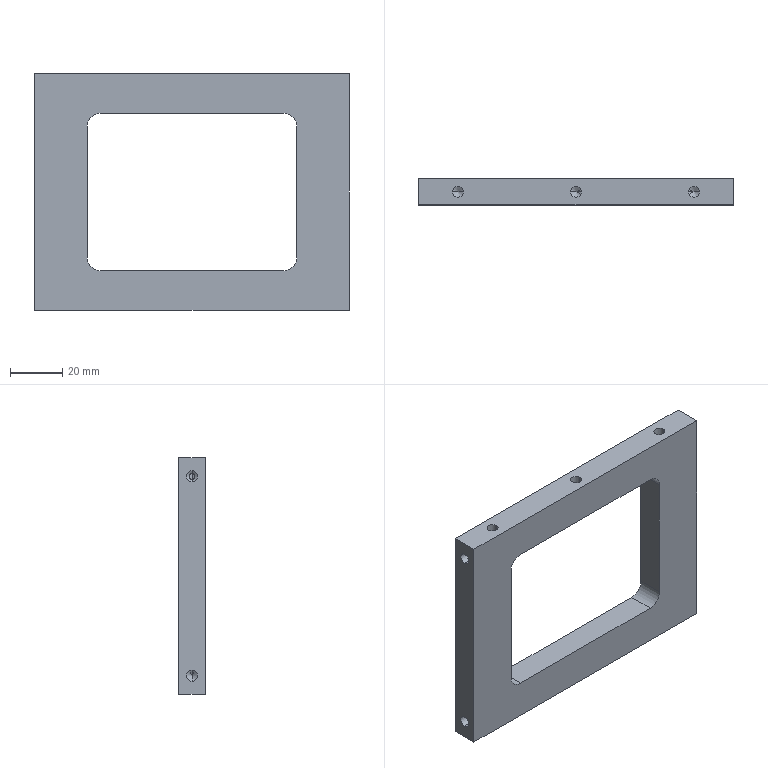Part | SolidWorks | features 3DProfileFeature 2, Cut 2, HoleWzd 2, Extrusion 1, ICE 1, MirrorPattern 1 | 1 solid | 42 faces | box 120 x 10 x 90 mm | volume 58973 mm3 | cylinder 18 | cone 14 | plane 10 | commonest cylinder face diameters 4.2 x14 10 x4
STEP:
#1=CARTESIAN_POINT('',(-45.,5.,31.338));
#2=VERTEX_POINT('',#1);
#3=CARTESIAN_POINT('',(-42.9,5.,32.6));
#4=VERTEX_POINT('',#3);
#5=CARTESIAN_POINT('',(-42.9,5.,32.6));
#6=DIRECTION('',(0.8572,0.,0.515));
#7=VECTOR('',#6,1000.);
#8=LINE('',#5,#7);
#9=EDGE_CURVE('',#2,#4,#8,.T.);
#10=ORIENTED_EDGE('',*,*,#9,.F.);
#11=CARTESIAN_POINT('',(-47.1,5.,32.6));
#12=VERTEX_POINT('',#11);
#13=CARTESIAN_POINT('',(-47.1,5.,32.6));
#14=DIRECTION('',(-0.8572,0.,0.515));
#15=VECTOR('',#14,1000.);
#16=LINE('',#13,#15);
#17=EDGE_CURVE('',#2,#12,#16,.T.);
#18=ORIENTED_EDGE('',*,*,#17,.T.);
#19=CARTESIAN_POINT('',(-45.,5.,32.6));
#20=DIRECTION('',(0.,0.,1.));
#21=DIRECTION('',(1.,0.,0.));
#22=AXIS2_PLACEMENT_3D('',#19,#20,#21);
#23=CIRCLE('',#22,2.1);
#24=EDGE_CURVE('',#12,#4,#23,.T.);
#25=ORIENTED_EDGE('',*,*,#24,.T.);
#26=EDGE_LOOP('',(#10,#18,#25));
#27=FACE_OUTER_BOUND('',#26,.T.);
#28=CARTESIAN_POINT('',(-45.,5.,32.6));
#29=DIRECTION('',(0.,0.,1.));
#30=DIRECTION('',(1.,0.,0.));
#31=AXIS2_PLACEMENT_3D('',#28,#29,#30);
#32=CONICAL_SURFACE('',#31,2.1,1.03);
#33=ADVANCED_FACE('',(#27),#32,.F.);
#34=ORIENTED_EDGE('',*,*,#24,.F.);
#35=CARTESIAN_POINT('',(-47.1,5.,36.732));
#36=VERTEX_POINT('',#35);
#37=CARTESIAN_POINT('',(-47.1,5.,45.));
#38=DIRECTION('',(0.,0.,1.));
#39=VECTOR('',#38,1000.);
#40=LINE('',#37,#39);
#41=EDGE_CURVE('',#12,#36,#40,.T.);
#42=ORIENTED_EDGE('',*,*,#41,.T.);
#43=CARTESIAN_POINT('',(-47.1,5.,39.268));
#44=VERTEX_POINT('',#43);
#45=CARTESIAN_POINT('',(-47.1,5.,39.268));
#46=CARTESIAN_POINT('',(-47.1,4.856,39.268));
#47=CARTESIAN_POINT('',(-47.084,4.712,39.214));
#48=CARTESIAN_POINT('',(-47.038,4.479,39.05));
#49=CARTESIAN_POINT('',(-47.009,4.383,38.94));
#50=CARTESIAN_POINT('',(-46.93,4.158,38.579));
#51=CARTESIAN_POINT('',(-46.889,4.083,38.287));
#52=CARTESIAN_POINT('',(-46.889,4.083,37.856));
#53=CARTESIAN_POINT('',(-46.899,4.102,37.71));
#54=CARTESIAN_POINT('',(-46.932,4.177,37.435));
#55=CARTESIAN_POINT('',(-46.956,4.233,37.301));
#56=CARTESIAN_POINT('',(-47.009,4.383,37.06));
#57=CARTESIAN_POINT('',(-47.038,4.478,36.95));
#58=CARTESIAN_POINT('',(-47.084,4.712,36.785));
#59=CARTESIAN_POINT('',(-47.1,4.856,36.732));
#60=CARTESIAN_POINT('',(-47.1,5.,36.732));
#61=B_SPLINE_CURVE_WITH_KNOTS('',3,(#45,#46,#47,#48,#49,#50,#51,#52,#53,#54,#55,#56,#57,#58,#59,#60),.UNSPECIFIED.,.F.,.F.,(4,2,2,2,2,2,2,4),(0.003814,0.004249,0.004683,0.005552,0.005986,0.00642,0.006854,0.007289),.UNSPECIFIED.);
#62=EDGE_CURVE('',#44,#36,#61,.T.);
#63=ORIENTED_EDGE('',*,*,#62,.F.);
#64=CARTESIAN_POINT('',(-47.1,5.,45.));
#65=VERTEX_POINT('',#64);
#66=CARTESIAN_POINT('',(-47.1,5.,45.));
#67=DIRECTION('',(0.,0.,1.));
#68=VECTOR('',#67,1000.);
#69=LINE('',#66,#68);
#70=EDGE_CURVE('',#44,#65,#69,.T.);
#71=ORIENTED_EDGE('',*,*,#70,.T.);
#72=CARTESIAN_POINT('',(-42.9,5.,45.));
#73=VERTEX_POINT('',#72);
#74=CARTESIAN_POINT('',(-45.,5.,45.));
#75=DIRECTION('',(0.,0.,1.));
#76=DIRECTION('',(1.,0.,0.));
#77=AXIS2_PLACEMENT_3D('',#74,#75,#76);
#78=CIRCLE('',#77,2.1);
#79=EDGE_CURVE('',#65,#73,#78,.T.);
#80=ORIENTED_EDGE('',*,*,#79,.T.);
#81=CARTESIAN_POINT('',(-42.9,5.,45.));
#82=DIRECTION('',(0.,0.,1.));
#83=VECTOR('',#82,1000.);
#84=LINE('',#81,#83);
#85=EDGE_CURVE('',#4,#73,#84,.T.);
#86=ORIENTED_EDGE('',*,*,#85,.F.);
#87=EDGE_LOOP('',(#34,#42,#63,#71,#80,#86));
#88=FACE_OUTER_BOUND('',#87,.T.);
#89=CARTESIAN_POINT('',(-45.,5.,45.));
#90=DIRECTION('',(0.,0.,1.));
#91=DIRECTION('',(1.,0.,0.));
#92=AXIS2_PLACEMENT_3D('',#89,#90,#91);
#93=CYLINDRICAL_SURFACE('',#92,2.1);
#94=ADVANCED_FACE('',(#88),#93,.F.);
#95=CARTESIAN_POINT('',(-2.1,5.,32.6));
#96=VERTEX_POINT('',#95);
#97=CARTESIAN_POINT('',(2.1,5.,32.6));
#98=VERTEX_POINT('',#97);
#99=CARTESIAN_POINT('',(0.,5.,32.6));
#100=DIRECTION('',(0.,0.,1.));
#101=DIRECTION('',(1.,0.,0.));
#102=AXIS2_PLACEMENT_3D('',#99,#100,#101);
#103=CIRCLE('',#102,2.1);
#104=EDGE_CURVE('',#96,#98,#103,.T.);
#105=ORIENTED_EDGE('',*,*,#104,.F.);
#106=CARTESIAN_POINT('',(-2.1,5.,45.));
#107=VERTEX_POINT('',#106);
#108=CARTESIAN_POINT('',(-2.1,5.,45.));
#109=DIRECTION('',(0.,0.,1.));
#110=VECTOR('',#109,1000.);
#111=LINE('',#108,#110);
#112=EDGE_CURVE('',#96,#107,#111,.T.);
#113=ORIENTED_EDGE('',*,*,#112,.T.);
#114=CARTESIAN_POINT('',(2.1,5.,45.));
#115=VERTEX_POINT('',#114);
#116=CARTESIAN_POINT('',(0.,5.,45.));
#117=DIRECTION('',(0.,0.,1.));
#118=DIRECTION('',(1.,0.,0.));
#119=AXIS2_PLACEMENT_3D('',#116,#117,#118);
#120=CIRCLE('',#119,2.1);
#121=EDGE_CURVE('',#107,#115,#120,.T.);
#122=ORIENTED_EDGE('',*,*,#121,.T.);
#123=CARTESIAN_POINT('',(2.1,5.,45.));
#124=DIRECTION('',(0.,0.,1.));
#125=VECTOR('',#124,1000.);
#126=LINE('',#123,#125);
#127=EDGE_CURVE('',#98,#115,#126,.T.);
#128=ORIENTED_EDGE('',*,*,#127,.F.);
#129=EDGE_LOOP('',(#105,#113,#122,#128));
#130=FACE_OUTER_BOUND('',#129,.T.);
#131=CARTESIAN_POINT('',(0.,5.,45.));
#132=DIRECTION('',(0.,0.,1.));
#133=DIRECTION('',(1.,0.,0.));
#134=AXIS2_PLACEMENT_3D('',#131,#132,#133);
#135=CYLINDRICAL_SURFACE('',#134,2.1);
#136=ADVANCED_FACE('',(#130),#135,.F.);
#137=CARTESIAN_POINT('',(0.,5.,31.338));
#138=VERTEX_POINT('',#137);
#139=CARTESIAN_POINT('',(2.1,5.,32.6));
#140=DIRECTION('',(0.8572,0.,0.515));
#141=VECTOR('',#140,1000.);
#142=LINE('',#139,#141);
#143=EDGE_CURVE('',#138,#98,#142,.T.);
#144=ORIENTED_EDGE('',*,*,#143,.F.);
#145=CARTESIAN_POINT('',(-2.1,5.,32.6));
#146=DIRECTION('',(-0.8572,0.,0.515));
#147=VECTOR('',#146,1000.);
#148=LINE('',#145,#147);
#149=EDGE_CURVE('',#138,#96,#148,.T.);
#150=ORIENTED_EDGE('',*,*,#149,.T.);
#151=ORIENTED_EDGE('',*,*,#104,.T.);
#152=EDGE_LOOP('',(#144,#150,#151));
#153=FACE_OUTER_BOUND('',#152,.T.);
#154=CARTESIAN_POINT('',(0.,5.,32.6));
#155=DIRECTION('',(0.,0.,1.));
#156=DIRECTION('',(1.,0.,0.));
#157=AXIS2_PLACEMENT_3D('',#154,#155,#156);
#158=CONICAL_SURFACE('',#157,2.1,1.03);
#159=ADVANCED_FACE('',(#153),#158,.F.);
#160=CARTESIAN_POINT('',(45.,5.,31.338));
#161=VERTEX_POINT('',#160);
#162=CARTESIAN_POINT('',(47.1,5.,32.6));
#163=VERTEX_POINT('',#162);
#164=CARTESIAN_POINT('',(47.1,5.,32.6));
#165=DIRECTION('',(0.8572,0.,0.515));
#166=VECTOR('',#165,1000.);
#167=LINE('',#164,#166);
#168=EDGE_CURVE('',#161,#163,#167,.T.);
#169=ORIENTED_EDGE('',*,*,#168,.F.);
#170=CARTESIAN_POINT('',(42.9,5.,32.6));
#171=VERTEX_POINT('',#170);
#172=CARTESIAN_POINT('',(42.9,5.,32.6));
#173=DIRECTION('',(-0.8572,0.,0.515));
#174=VECTOR('',#173,1000.);
#175=LINE('',#172,#174);
#176=EDGE_CURVE('',#161,#171,#175,.T.);
#177=ORIENTED_EDGE('',*,*,#176,.T.);
#178=CARTESIAN_POINT('',(45.,5.,32.6));
#179=DIRECTION('',(0.,0.,1.));
#180=DIRECTION('',(1.,0.,0.));
#181=AXIS2_PLACEMENT_3D('',#178,#179,#180);
#182=CIRCLE('',#181,2.1);
#183=EDGE_CURVE('',#171,#163,#182,.T.);
#184=ORIENTED_EDGE('',*,*,#183,.T.);
#185=EDGE_LOOP('',(#169,#177,#184));
#186=FACE_OUTER_BOUND('',#185,.T.);
#187=CARTESIAN_POINT('',(45.,5.,32.6));
#188=DIRECTION('',(0.,0.,1.));
#189=DIRECTION('',(1.,0.,0.));
#190=AXIS2_PLACEMENT_3D('',#187,#188,#189);
#191=CONICAL_SURFACE('',#190,2.1,1.03);
#192=ADVANCED_FACE('',(#186),#191,.F.);
#193=ORIENTED_EDGE('',*,*,#183,.F.);
#194=CARTESIAN_POINT('',(42.9,5.,45.));
#195=VERTEX_POINT('',#194);
#196=CARTESIAN_POINT('',(42.9,5.,45.));
#197=DIRECTION('',(0.,0.,1.));
#198=VECTOR('',#197,1000.);
#199=LINE('',#196,#198);
#200=EDGE_CURVE('',#171,#195,#199,.T.);
#201=ORIENTED_EDGE('',*,*,#200,.T.);
#202=CARTESIAN_POINT('',(47.1,5.,45.));
#203=VERTEX_POINT('',#202);
#204=CARTESIAN_POINT('',(45.,5.,45.));
#205=DIRECTION('',(0.,0.,1.));
#206=DIRECTION('',(1.,0.,0.));
#207=AXIS2_PLACEMENT_3D('',#204,#205,#206);
#208=CIRCLE('',#207,2.1);
#209=EDGE_CURVE('',#195,#203,#208,.T.);
#210=ORIENTED_EDGE('',*,*,#209,.T.);
#211=CARTESIAN_POINT('',(47.1,5.,39.268));
#212=VERTEX_POINT('',#211);
#213=CARTESIAN_POINT('',(47.1,5.,45.));
#214=DIRECTION('',(0.,0.,1.));
#215=VECTOR('',#214,1000.);
#216=LINE('',#213,#215);
#217=EDGE_CURVE('',#212,#203,#216,.T.);
#218=ORIENTED_EDGE('',*,*,#217,.F.);
#219=CARTESIAN_POINT('',(47.1,5.,36.732));
#220=VERTEX_POINT('',#219);
#221=CARTESIAN_POINT('',(47.1,5.,36.732));
#222=CARTESIAN_POINT('',(47.1,4.855,36.732));
#223=CARTESIAN_POINT('',(47.083,4.711,36.786));
#224=CARTESIAN_POINT('',(47.038,4.478,36.95));
#225=CARTESIAN_POINT('',(47.009,4.383,37.06));
#226=CARTESIAN_POINT('',(46.93,4.158,37.421));
#227=CARTESIAN_POINT('',(46.889,4.083,37.713));
#228=CARTESIAN_POINT('',(46.889,4.083,38.145));
#229=CARTESIAN_POINT('',(46.899,4.102,38.289));
#230=CARTESIAN_POINT('',(46.932,4.177,38.566));
#231=CARTESIAN_POINT('',(46.956,4.232,38.698));
#232=CARTESIAN_POINT('',(47.009,4.383,38.941));
#233=CARTESIAN_POINT('',(47.038,4.478,39.05));
#234=CARTESIAN_POINT('',(47.084,4.712,39.214));
#235=CARTESIAN_POINT('',(47.1,4.855,39.268));
#236=CARTESIAN_POINT('',(47.1,5.,39.268));
#237=B_SPLINE_CURVE_WITH_KNOTS('',3,(#221,#222,#223,#224,#225,#226,#227,#228,#229,#230,#231,#232,#233,#234,#235,#236),.UNSPECIFIED.,.F.,.F.,(4,2,2,2,2,2,2,4),(0.006577,0.007009,0.007441,0.008306,0.008738,0.00917,0.009602,0.01003),.UNSPECIFIED.);
#238=EDGE_CURVE('',#220,#212,#237,.T.);
#239=ORIENTED_EDGE('',*,*,#238,.F.);
#240=CARTESIAN_POINT('',(47.1,5.,45.));
#241=DIRECTION('',(0.,0.,1.));
#242=VECTOR('',#241,1000.);
#243=LINE('',#240,#242);
#244=EDGE_CURVE('',#163,#220,#243,.T.);
#245=ORIENTED_EDGE('',*,*,#244,.F.);
#246=EDGE_LOOP('',(#193,#201,#210,#218,#239,#245));
#247=FACE_OUTER_BOUND('',#246,.T.);
#248=CARTESIAN_POINT('',(45.,5.,45.));
#249=DIRECTION('',(0.,0.,1.));
#250=DIRECTION('',(1.,0.,0.));
#251=AXIS2_PLACEMENT_3D('',#248,#249,#250);
#252=CYLINDRICAL_SURFACE('',#251,2.1);
#253=ADVANCED_FACE('',(#247),#252,.F.);
#254=CARTESIAN_POINT('',(47.6,5.,40.1));
#255=VERTEX_POINT('',#254);
#256=CARTESIAN_POINT('',(47.6,5.,35.9));
#257=VERTEX_POINT('',#256);
#258=CARTESIAN_POINT('',(47.6,5.,38.));
#259=DIRECTION('',(1.,0.,0.));
#260=DIRECTION('',(0.,0.,-1.));
#261=AXIS2_PLACEMENT_3D('',#258,#259,#260);
#262=CIRCLE('',#261,2.1);
#263=EDGE_CURVE('',#255,#257,#262,.T.);
#264=ORIENTED_EDGE('',*,*,#263,.F.);
#265=CARTESIAN_POINT('',(60.,5.,40.1));
#266=VERTEX_POINT('',#265);
#267=CARTESIAN_POINT('',(60.,5.,40.1));
#268=DIRECTION('',(1.,0.,0.));
#269=VECTOR('',#268,1000.);
#270=LINE('',#267,#269);
#271=EDGE_CURVE('',#255,#266,#270,.T.);
#272=ORIENTED_EDGE('',*,*,#271,.T.);
#273=CARTESIAN_POINT('',(60.,5.,35.9));
#274=VERTEX_POINT('',#273);
#275=CARTESIAN_POINT('',(60.,5.,38.));
#276=DIRECTION('',(1.,0.,0.));
#277=DIRECTION('',(0.,0.,-1.));
#278=AXIS2_PLACEMENT_3D('',#275,#276,#277);
#279=CIRCLE('',#278,2.1);
#280=EDGE_CURVE('',#266,#274,#279,.T.);
#281=ORIENTED_EDGE('',*,*,#280,.T.);
#282=CARTESIAN_POINT('',(60.,5.,35.9));
#283=DIRECTION('',(1.,0.,0.));
#284=VECTOR('',#283,1000.);
#285=LINE('',#282,#284);
#286=EDGE_CURVE('',#257,#274,#285,.T.);
#287=ORIENTED_EDGE('',*,*,#286,.F.);
#288=EDGE_LOOP('',(#264,#272,#281,#287));
#289=FACE_OUTER_BOUND('',#288,.T.);
#290=CARTESIAN_POINT('',(60.,5.,38.));
#291=DIRECTION('',(1.,0.,0.));
#292=DIRECTION('',(0.,0.,-1.));
#293=AXIS2_PLACEMENT_3D('',#290,#291,#292);
#294=CYLINDRICAL_SURFACE('',#293,2.1);
#295=ADVANCED_FACE('',(#289),#294,.F.);
#296=ORIENTED_EDGE('',*,*,#238,.T.);
#297=CARTESIAN_POINT('',(47.6,5.,40.1));
#298=DIRECTION('',(0.515,0.,0.8572));
#299=VECTOR('',#298,1000.);
#300=LINE('',#297,#299);
#301=EDGE_CURVE('',#212,#255,#300,.T.);
#302=ORIENTED_EDGE('',*,*,#301,.T.);
#303=ORIENTED_EDGE('',*,*,#263,.T.);
#304=CARTESIAN_POINT('',(47.6,5.,35.9));
#305=DIRECTION('',(0.515,0.,-0.8572));
#306=VECTOR('',#305,1000.);
#307=LINE('',#304,#306);
#308=EDGE_CURVE('',#220,#257,#307,.T.);
#309=ORIENTED_EDGE('',*,*,#308,.F.);
#310=EDGE_LOOP('',(#296,#302,#303,#309));
#311=FACE_OUTER_BOUND('',#310,.T.);
#312=CARTESIAN_POINT('',(47.6,5.,38.));
#313=DIRECTION('',(1.,0.,0.));
#314=DIRECTION('',(0.,0.,-1.));
#315=AXIS2_PLACEMENT_3D('',#312,#313,#314);
#316=CONICAL_SURFACE('',#315,2.1,1.03);
#317=ADVANCED_FACE('',(#311),#316,.F.);
#318=CARTESIAN_POINT('',(47.6,5.,-35.9));
#319=VERTEX_POINT('',#318);
#320=CARTESIAN_POINT('',(47.6,5.,-40.1));
#321=VERTEX_POINT('',#320);
#322=CARTESIAN_POINT('',(47.6,5.,-38.));
#323=DIRECTION('',(1.,0.,0.));
#324=DIRECTION('',(0.,0.,-1.));
#325=AXIS2_PLACEMENT_3D('',#322,#323,#324);
#326=CIRCLE('',#325,2.1);
#327=EDGE_CURVE('',#319,#321,#326,.T.);
#328=ORIENTED_EDGE('',*,*,#327,.F.);
#329=CARTESIAN_POINT('',(60.,5.,-35.9));
#330=VERTEX_POINT('',#329);
#331=CARTESIAN_POINT('',(60.,5.,-35.9));
#332=DIRECTION('',(1.,0.,0.));
#333=VECTOR('',#332,1000.);
#334=LINE('',#331,#333);
#335=EDGE_CURVE('',#319,#330,#334,.T.);
#336=ORIENTED_EDGE('',*,*,#335,.T.);
#337=CARTESIAN_POINT('',(60.,5.,-40.1));
#338=VERTEX_POINT('',#337);
#339=CARTESIAN_POINT('',(60.,5.,-38.));
#340=DIRECTION('',(1.,0.,0.));
#341=DIRECTION('',(0.,0.,-1.));
#342=AXIS2_PLACEMENT_3D('',#339,#340,#341);
#343=CIRCLE('',#342,2.1);
#344=EDGE_CURVE('',#330,#338,#343,.T.);
#345=ORIENTED_EDGE('',*,*,#344,.T.);
#346=CARTESIAN_POINT('',(60.,5.,-40.1));
#347=DIRECTION('',(1.,0.,0.));
#348=VECTOR('',#347,1000.);
#349=LINE('',#346,#348);
#350=EDGE_CURVE('',#321,#338,#349,.T.);
#351=ORIENTED_EDGE('',*,*,#350,.F.);
#352=EDGE_LOOP('',(#328,#336,#345,#351));
#353=FACE_OUTER_BOUND('',#352,.T.);
#354=CARTESIAN_POINT('',(60.,5.,-38.));
#355=DIRECTION('',(1.,0.,0.));
#356=DIRECTION('',(0.,0.,-1.));
#357=AXIS2_PLACEMENT_3D('',#354,#355,#356);
#358=CYLINDRICAL_SURFACE('',#357,2.1);
#359=ADVANCED_FACE('',(#353),#358,.F.);
#360=CARTESIAN_POINT('',(46.338,5.,-38.));
#361=VERTEX_POINT('',#360);
#362=CARTESIAN_POINT('',(47.6,5.,-40.1));
#363=DIRECTION('',(0.515,0.,-0.8572));
#364=VECTOR('',#363,1000.);
#365=LINE('',#362,#364);
#366=EDGE_CURVE('',#361,#321,#365,.T.);
#367=ORIENTED_EDGE('',*,*,#366,.F.);
#368=CARTESIAN_POINT('',(47.6,5.,-35.9));
#369=DIRECTION('',(0.515,0.,0.8572));
#370=VECTOR('',#369,1000.);
#371=LINE('',#368,#370);
#372=EDGE_CURVE('',#361,#319,#371,.T.);
#373=ORIENTED_EDGE('',*,*,#372,.T.);
#374=ORIENTED_EDGE('',*,*,#327,.T.);
#375=EDGE_LOOP('',(#367,#373,#374));
#376=FACE_OUTER_BOUND('',#375,.T.);
#377=CARTESIAN_POINT('',(47.6,5.,-38.));
#378=DIRECTION('',(1.,0.,0.));
#379=DIRECTION('',(0.,0.,-1.));
#380=AXIS2_PLACEMENT_3D('',#377,#378,#379);
#381=CONICAL_SURFACE('',#380,2.1,1.03);
#382=ADVANCED_FACE('',(#376),#381,.F.);
#383=CARTESIAN_POINT('',(-47.6,5.,35.9));
#384=VERTEX_POINT('',#383);
#385=CARTESIAN_POINT('',(-47.6,5.,40.1));
#386=VERTEX_POINT('',#385);
#387=CARTESIAN_POINT('',(-47.6,5.,38.));
#388=DIRECTION('',(-1.,0.,0.));
#389=DIRECTION('',(0.,0.,1.));
#390=AXIS2_PLACEMENT_3D('',#387,#388,#389);
#391=CIRCLE('',#390,2.1);
#392=EDGE_CURVE('',#384,#386,#391,.T.);
#393=ORIENTED_EDGE('',*,*,#392,.F.);
#394=CARTESIAN_POINT('',(-60.,5.,35.9));
#395=VERTEX_POINT('',#394);
#396=CARTESIAN_POINT('',(-60.,5.,35.9));
#397=DIRECTION('',(-1.,0.,0.));
#398=VECTOR('',#397,1000.);
#399=LINE('',#396,#398);
#400=EDGE_CURVE('',#384,#395,#399,.T.);
#401=ORIENTED_EDGE('',*,*,#400,.T.);
#402=CARTESIAN_POINT('',(-60.,5.,40.1));
#403=VERTEX_POINT('',#402);
#404=CARTESIAN_POINT('',(-60.,5.,38.));
#405=DIRECTION('',(-1.,0.,0.));
#406=DIRECTION('',(0.,0.,1.));
#407=AXIS2_PLACEMENT_3D('',#404,#405,#406);
#408=CIRCLE('',#407,2.1);
#409=EDGE_CURVE('',#395,#403,#408,.T.);
#410=ORIENTED_EDGE('',*,*,#409,.T.);
#411=CARTESIAN_POINT('',(-60.,5.,40.1));
#412=DIRECTION('',(-1.,0.,0.));
#413=VECTOR('',#412,1000.);
#414=LINE('',#411,#413);
#415=EDGE_CURVE('',#386,#403,#414,.T.);
#416=ORIENTED_EDGE('',*,*,#415,.F.);
#417=EDGE_LOOP('',(#393,#401,#410,#416));
#418=FACE_OUTER_BOUND('',#417,.T.);
#419=CARTESIAN_POINT('',(-60.,5.,38.));
#420=DIRECTION('',(-1.,0.,0.));
#421=DIRECTION('',(0.,0.,1.));
#422=AXIS2_PLACEMENT_3D('',#419,#420,#421);
#423=CYLINDRICAL_SURFACE('',#422,2.1);
#424=ADVANCED_FACE('',(#418),#423,.F.);
#425=ORIENTED_EDGE('',*,*,#62,.T.);
#426=CARTESIAN_POINT('',(-47.6,5.,35.9));
#427=DIRECTION('',(-0.515,0.,-0.8572));
#428=VECTOR('',#427,1000.);
#429=LINE('',#426,#428);
#430=EDGE_CURVE('',#36,#384,#429,.T.);
#431=ORIENTED_EDGE('',*,*,#430,.T.);
#432=ORIENTED_EDGE('',*,*,#392,.T.);
#433=CARTESIAN_POINT('',(-47.6,5.,40.1));
#434=DIRECTION('',(-0.515,0.,0.8572));
#435=VECTOR('',#434,1000.);
#436=LINE('',#433,#435);
#437=EDGE_CURVE('',#44,#386,#436,.T.);
#438=ORIENTED_EDGE('',*,*,#437,.F.);
#439=EDGE_LOOP('',(#425,#431,#432,#438));
#440=FACE_OUTER_BOUND('',#439,.T.);
#441=CARTESIAN_POINT('',(-47.6,5.,38.));
#442=DIRECTION('',(-1.,0.,0.));
#443=DIRECTION('',(0.,0.,1.));
#444=AXIS2_PLACEMENT_3D('',#441,#442,#443);
#445=CONICAL_SURFACE('',#444,2.1,1.03);
#446=ADVANCED_FACE('',(#440),#445,.F.);
#447=CARTESIAN_POINT('',(-47.6,5.,-40.1));
#448=VERTEX_POINT('',#447);
#449=CARTESIAN_POINT('',(-47.6,5.,-35.9));
#450=VERTEX_POINT('',#449);
#451=CARTESIAN_POINT('',(-47.6,5.,-38.));
#452=DIRECTION('',(-1.,0.,0.));
#453=DIRECTION('',(0.,0.,1.));
#454=AXIS2_PLACEMENT_3D('',#451,#452,#453);
#455=CIRCLE('',#454,2.1);
#456=EDGE_CURVE('',#448,#450,#455,.T.);
#457=ORIENTED_EDGE('',*,*,#456,.F.);
#458=CARTESIAN_POINT('',(-60.,5.,-40.1));
#459=VERTEX_POINT('',#458);
#460=CARTESIAN_POINT('',(-60.,5.,-40.1));
#461=DIRECTION('',(-1.,0.,0.));
#462=VECTOR('',#461,1000.);
#463=LINE('',#460,#462);
#464=EDGE_CURVE('',#448,#459,#463,.T.);
#465=ORIENTED_EDGE('',*,*,#464,.T.);
#466=CARTESIAN_POINT('',(-60.,5.,-35.9));
#467=VERTEX_POINT('',#466);
#468=CARTESIAN_POINT('',(-60.,5.,-38.));
#469=DIRECTION('',(-1.,0.,0.));
#470=DIRECTION('',(0.,0.,1.));
#471=AXIS2_PLACEMENT_3D('',#468,#469,#470);
#472=CIRCLE('',#471,2.1);
#473=EDGE_CURVE('',#459,#467,#472,.T.);
#474=ORIENTED_EDGE('',*,*,#473,.T.);
#475=CARTESIAN_POINT('',(-60.,5.,-35.9));
#476=DIRECTION('',(-1.,0.,0.));
#477=VECTOR('',#476,1000.);
#478=LINE('',#475,#477);
#479=EDGE_CURVE('',#450,#467,#478,.T.);
#480=ORIENTED_EDGE('',*,*,#479,.F.);
#481=EDGE_LOOP('',(#457,#465,#474,#480));
#482=FACE_OUTER_BOUND('',#481,.T.);
#483=CARTESIAN_POINT('',(-60.,5.,-38.));
#484=DIRECTION('',(-1.,0.,0.));
#485=DIRECTION('',(0.,0.,1.));
#486=AXIS2_PLACEMENT_3D('',#483,#484,#485);
#487=CYLINDRICAL_SURFACE('',#486,2.1);
#488=ADVANCED_FACE('',(#482),#487,.F.);
#489=CARTESIAN_POINT('',(-46.338,5.,-38.));
#490=VERTEX_POINT('',#489);
#491=CARTESIAN_POINT('',(-47.6,5.,-35.9));
#492=DIRECTION('',(-0.515,0.,0.8572));
#493=VECTOR('',#492,1000.);
#494=LINE('',#491,#493);
#495=EDGE_CURVE('',#490,#450,#494,.T.);
#496=ORIENTED_EDGE('',*,*,#495,.F.);
#497=CARTESIAN_POINT('',(-47.6,5.,-40.1));
#498=DIRECTION('',(-0.515,0.,-0.8572));
#499=VECTOR('',#498,1000.);
#500=LINE('',#497,#499);
#501=EDGE_CURVE('',#490,#448,#500,.T.);
#502=ORIENTED_EDGE('',*,*,#501,.T.);
#503=ORIENTED_EDGE('',*,*,#456,.T.);
#504=EDGE_LOOP('',(#496,#502,#503));
#505=FACE_OUTER_BOUND('',#504,.T.);
#506=CARTESIAN_POINT('',(-47.6,5.,-38.));
#507=DIRECTION('',(-1.,0.,0.));
#508=DIRECTION('',(0.,0.,1.));
#509=AXIS2_PLACEMENT_3D('',#506,#507,#508);
#510=CONICAL_SURFACE('',#509,2.1,1.03);
#511=ADVANCED_FACE('',(#505),#510,.F.);
#512=CARTESIAN_POINT('',(60.,5.,38.));
#513=DIRECTION('',(1.,0.,0.));
#514=DIRECTION('',(0.,0.,-1.));
#515=AXIS2_PLACEMENT_3D('',#512,#513,#514);
#516=CIRCLE('',#515,2.1);
#517=EDGE_CURVE('',#274,#266,#516,.T.);
#518=ORIENTED_EDGE('',*,*,#517,.F.);
#519=ORIENTED_EDGE('',*,*,#280,.F.);
#520=EDGE_LOOP('',(#518,#519));
#521=FACE_BOUND('',#520,.T.);
#522=CARTESIAN_POINT('',(60.,5.,-38.));
#523=DIRECTION('',(1.,0.,0.));
#524=DIRECTION('',(0.,0.,-1.));
#525=AXIS2_PLACEMENT_3D('',#522,#523,#524);
#526=CIRCLE('',#525,2.1);
#527=EDGE_CURVE('',#338,#330,#526,.T.);
#528=ORIENTED_EDGE('',*,*,#527,.F.);
#529=ORIENTED_EDGE('',*,*,#344,.F.);
#530=EDGE_LOOP('',(#528,#529));
#531=FACE_BOUND('',#530,.T.);
#532=CARTESIAN_POINT('',(60.,0.,45.));
#533=VERTEX_POINT('',#532);
#534=CARTESIAN_POINT('',(60.,0.,-45.));
#535=VERTEX_POINT('',#534);
#536=CARTESIAN_POINT('',(60.,0.,-45.));
#537=DIRECTION('',(0.,0.,-1.));
#538=VECTOR('',#537,1000.);
#539=LINE('',#536,#538);
#540=EDGE_CURVE('',#533,#535,#539,.T.);
#541=ORIENTED_EDGE('',*,*,#540,.T.);
#542=CARTESIAN_POINT('',(60.,10.,-45.));
#543=VERTEX_POINT('',#542);
#544=CARTESIAN_POINT('',(60.,10.,-45.));
#545=DIRECTION('',(0.,-1.,0.));
#546=VECTOR('',#545,1000.);
#547=LINE('',#544,#546);
#548=EDGE_CURVE('',#543,#535,#547,.T.);
#549=ORIENTED_EDGE('',*,*,#548,.F.);
#550=CARTESIAN_POINT('',(60.,10.,45.));
#551=VERTEX_POINT('',#550);
#552=CARTESIAN_POINT('',(60.,10.,-45.));
#553=DIRECTION('',(0.,0.,-1.));
#554=VECTOR('',#553,1000.);
#555=LINE('',#552,#554);
#556=EDGE_CURVE('',#551,#543,#555,.T.);
#557=ORIENTED_EDGE('',*,*,#556,.F.);
#558=CARTESIAN_POINT('',(60.,10.,45.));
#559=DIRECTION('',(0.,-1.,0.));
#560=VECTOR('',#559,1000.);
#561=LINE('',#558,#560);
#562=EDGE_CURVE('',#551,#533,#561,.T.);
#563=ORIENTED_EDGE('',*,*,#562,.T.);
#564=EDGE_LOOP('',(#541,#549,#557,#563));
#565=FACE_OUTER_BOUND('',#564,.T.);
#566=CARTESIAN_POINT('',(60.,10.,-45.));
#567=DIRECTION('',(-1.,0.,0.));
#568=DIRECTION('',(0.,0.,1.));
#569=AXIS2_PLACEMENT_3D('',#566,#567,#568);
#570=PLANE('',#569);
#571=ADVANCED_FACE('',(#521,#531,#565),#570,.F.);
#572=CARTESIAN_POINT('',(-60.,0.,-45.));
#573=VERTEX_POINT('',#572);
#574=CARTESIAN_POINT('',(-60.,0.,-45.));
#575=DIRECTION('',(-1.,0.,0.));
#576=VECTOR('',#575,1000.);
#577=LINE('',#574,#576);
#578=EDGE_CURVE('',#535,#573,#577,.T.);
#579=ORIENTED_EDGE('',*,*,#578,.T.);
#580=CARTESIAN_POINT('',(-60.,10.,-45.));
#581=VERTEX_POINT('',#580);
#582=CARTESIAN_POINT('',(-60.,10.,-45.));
#583=DIRECTION('',(0.,-1.,0.));
#584=VECTOR('',#583,1000.);
#585=LINE('',#582,#584);
#586=EDGE_CURVE('',#581,#573,#585,.T.);
#587=ORIENTED_EDGE('',*,*,#586,.F.);
#588=CARTESIAN_POINT('',(-60.,10.,-45.));
#589=DIRECTION('',(-1.,0.,0.));
#590=VECTOR('',#589,1000.);
#591=LINE('',#588,#590);
#592=EDGE_CURVE('',#543,#581,#591,.T.);
#593=ORIENTED_EDGE('',*,*,#592,.F.);
#594=ORIENTED_EDGE('',*,*,#548,.T.);
#595=EDGE_LOOP('',(#579,#587,#593,#594));
#596=FACE_OUTER_BOUND('',#595,.T.);
#597=CARTESIAN_POINT('',(-60.,10.,-45.));
#598=DIRECTION('',(0.,0.,1.));
#599=DIRECTION('',(1.,0.,0.));
#600=AXIS2_PLACEMENT_3D('',#597,#598,#599);
#601=PLANE('',#600);
#602=ADVANCED_FACE('',(#596),#601,.F.);
#603=CARTESIAN_POINT('',(-60.,5.,38.));
#604=DIRECTION('',(-1.,0.,0.));
#605=DIRECTION('',(0.,0.,1.));
#606=AXIS2_PLACEMENT_3D('',#603,#604,#605);
#607=CIRCLE('',#606,2.1);
#608=EDGE_CURVE('',#403,#395,#607,.T.);
#609=ORIENTED_EDGE('',*,*,#608,.F.);
#610=ORIENTED_EDGE('',*,*,#409,.F.);
#611=EDGE_LOOP('',(#609,#610));
#612=FACE_BOUND('',#611,.T.);
#613=CARTESIAN_POINT('',(-60.,5.,-38.));
#614=DIRECTION('',(-1.,0.,0.));
#615=DIRECTION('',(0.,0.,1.));
#616=AXIS2_PLACEMENT_3D('',#613,#614,#615);
#617=CIRCLE('',#616,2.1);
#618=EDGE_CURVE('',#467,#459,#617,.T.);
#619=ORIENTED_EDGE('',*,*,#618,.F.);
#620=ORIENTED_EDGE('',*,*,#473,.F.);
#621=EDGE_LOOP('',(#619,#620));
#622=FACE_BOUND('',#621,.T.);
#623=CARTESIAN_POINT('',(-60.,0.,45.));
#624=VERTEX_POINT('',#623);
#625=CARTESIAN_POINT('',(-60.,0.,-45.));
#626=DIRECTION('',(0.,0.,1.));
#627=VECTOR('',#626,1000.);
#628=LINE('',#625,#627);
#629=EDGE_CURVE('',#573,#624,#628,.T.);
#630=ORIENTED_EDGE('',*,*,#629,.T.);
#631=CARTESIAN_POINT('',(-60.,10.,45.));
#632=VERTEX_POINT('',#631);
#633=CARTESIAN_POINT('',(-60.,10.,45.));
#634=DIRECTION('',(0.,-1.,0.));
#635=VECTOR('',#634,1000.);
#636=LINE('',#633,#635);
#637=EDGE_CURVE('',#632,#624,#636,.T.);
#638=ORIENTED_EDGE('',*,*,#637,.F.);
#639=CARTESIAN_POINT('',(-60.,10.,-45.));
#640=DIRECTION('',(0.,0.,1.));
#641=VECTOR('',#640,1000.);
#642=LINE('',#639,#641);
#643=EDGE_CURVE('',#581,#632,#642,.T.);
#644=ORIENTED_EDGE('',*,*,#643,.F.);
#645=ORIENTED_EDGE('',*,*,#586,.T.);
#646=EDGE_LOOP('',(#630,#638,#644,#645));
#647=FACE_OUTER_BOUND('',#646,.T.);
#648=CARTESIAN_POINT('',(-60.,10.,-45.));
#649=DIRECTION('',(1.,0.,0.));
#650=DIRECTION('',(0.,0.,-1.));
#651=AXIS2_PLACEMENT_3D('',#648,#649,#650);
#652=PLANE('',#651);
#653=ADVANCED_FACE('',(#612,#622,#647),#652,.F.);
#654=CARTESIAN_POINT('',(-45.,5.,45.));
#655=DIRECTION('',(0.,0.,1.));
#656=DIRECTION('',(1.,0.,0.));
#657=AXIS2_PLACEMENT_3D('',#654,#655,#656);
#658=CIRCLE('',#657,2.1);
#659=EDGE_CURVE('',#73,#65,#658,.T.);
#660=ORIENTED_EDGE('',*,*,#659,.F.);
#661=ORIENTED_EDGE('',*,*,#79,.F.);
#662=EDGE_LOOP('',(#660,#661));
#663=FACE_BOUND('',#662,.T.);
#664=CARTESIAN_POINT('',(0.,5.,45.));
#665=DIRECTION('',(0.,0.,1.));
#666=DIRECTION('',(1.,0.,0.));
#667=AXIS2_PLACEMENT_3D('',#664,#665,#666);
#668=CIRCLE('',#667,2.1);
#669=EDGE_CURVE('',#115,#107,#668,.T.);
#670=ORIENTED_EDGE('',*,*,#669,.F.);
#671=ORIENTED_EDGE('',*,*,#121,.F.);
#672=EDGE_LOOP('',(#670,#671));
#673=FACE_BOUND('',#672,.T.);
#674=CARTESIAN_POINT('',(45.,5.,45.));
#675=DIRECTION('',(0.,0.,1.));
#676=DIRECTION('',(1.,0.,0.));
#677=AXIS2_PLACEMENT_3D('',#674,#675,#676);
#678=CIRCLE('',#677,2.1);
#679=EDGE_CURVE('',#203,#195,#678,.T.);
#680=ORIENTED_EDGE('',*,*,#679,.F.);
#681=ORIENTED_EDGE('',*,*,#209,.F.);
#682=EDGE_LOOP('',(#680,#681));
#683=FACE_BOUND('',#682,.T.);
#684=CARTESIAN_POINT('',(-60.,0.,45.));
#685=DIRECTION('',(1.,0.,0.));
#686=VECTOR('',#685,1000.);
#687=LINE('',#684,#686);
#688=EDGE_CURVE('',#624,#533,#687,.T.);
#689=ORIENTED_EDGE('',*,*,#688,.T.);
#690=ORIENTED_EDGE('',*,*,#562,.F.);
#691=CARTESIAN_POINT('',(-60.,10.,45.));
#692=DIRECTION('',(1.,0.,0.));
#693=VECTOR('',#692,1000.);
#694=LINE('',#691,#693);
#695=EDGE_CURVE('',#632,#551,#694,.T.);
#696=ORIENTED_EDGE('',*,*,#695,.F.);
#697=ORIENTED_EDGE('',*,*,#637,.T.);
#698=EDGE_LOOP('',(#689,#690,#696,#697));
#699=FACE_OUTER_BOUND('',#698,.T.);
#700=CARTESIAN_POINT('',(-60.,10.,45.));
#701=DIRECTION('',(0.,0.,-1.));
#702=DIRECTION('',(-1.,0.,0.));
#703=AXIS2_PLACEMENT_3D('',#700,#701,#702);
#704=PLANE('',#703);
#705=ADVANCED_FACE('',(#663,#673,#683,#699),#704,.F.);
#706=CARTESIAN_POINT('',(-40.,10.,-25.));
#707=VERTEX_POINT('',#706);
#708=CARTESIAN_POINT('',(-35.,10.,-30.));
#709=VERTEX_POINT('',#708);
#710=CARTESIAN_POINT('',(-35.,10.,-25.));
#711=DIRECTION('',(0.,-1.,0.));
#712=DIRECTION('',(0.,0.,-1.));
#713=AXIS2_PLACEMENT_3D('',#710,#711,#712);
#714=CIRCLE('',#713,5.);
#715=EDGE_CURVE('',#707,#709,#714,.T.);
#716=ORIENTED_EDGE('',*,*,#715,.T.);
#717=CARTESIAN_POINT('',(35.,10.,-30.));
#718=VERTEX_POINT('',#717);
#719=CARTESIAN_POINT('',(-35.,10.,-30.));
#720=DIRECTION('',(1.,0.,0.));
#721=VECTOR('',#720,1000.);
#722=LINE('',#719,#721);
#723=EDGE_CURVE('',#709,#718,#722,.T.);
#724=ORIENTED_EDGE('',*,*,#723,.T.);
#725=CARTESIAN_POINT('',(40.,10.,-25.));
#726=VERTEX_POINT('',#725);
#727=CARTESIAN_POINT('',(35.,10.,-25.));
#728=DIRECTION('',(0.,-1.,0.));
#729=DIRECTION('',(0.,0.,-1.));
#730=AXIS2_PLACEMENT_3D('',#727,#728,#729);
#731=CIRCLE('',#730,5.);
#732=EDGE_CURVE('',#718,#726,#731,.T.);
#733=ORIENTED_EDGE('',*,*,#732,.T.);
#734=CARTESIAN_POINT('',(40.,10.,25.));
#735=VERTEX_POINT('',#734);
#736=CARTESIAN_POINT('',(40.,10.,25.));
#737=DIRECTION('',(0.,0.,1.));
#738=VECTOR('',#737,1000.);
#739=LINE('',#736,#738);
#740=EDGE_CURVE('',#726,#735,#739,.T.);
#741=ORIENTED_EDGE('',*,*,#740,.T.);
#742=CARTESIAN_POINT('',(35.,10.,30.));
#743=VERTEX_POINT('',#742);
#744=CARTESIAN_POINT('',(35.,10.,25.));
#745=DIRECTION('',(0.,-1.,0.));
#746=DIRECTION('',(0.,0.,-1.));
#747=AXIS2_PLACEMENT_3D('',#744,#745,#746);
#748=CIRCLE('',#747,5.);
#749=EDGE_CURVE('',#735,#743,#748,.T.);
#750=ORIENTED_EDGE('',*,*,#749,.T.);
#751=CARTESIAN_POINT('',(-35.,10.,30.));
#752=VERTEX_POINT('',#751);
#753=CARTESIAN_POINT('',(-35.,10.,30.));
#754=DIRECTION('',(-1.,0.,0.));
#755=VECTOR('',#754,1000.);
#756=LINE('',#753,#755);
#757=EDGE_CURVE('',#743,#752,#756,.T.);
#758=ORIENTED_EDGE('',*,*,#757,.T.);
#759=CARTESIAN_POINT('',(-40.,10.,25.));
#760=VERTEX_POINT('',#759);
#761=CARTESIAN_POINT('',(-35.,10.,25.));
#762=DIRECTION('',(0.,-1.,0.));
#763=DIRECTION('',(0.,0.,-1.));
#764=AXIS2_PLACEMENT_3D('',#761,#762,#763);
#765=CIRCLE('',#764,5.);
#766=EDGE_CURVE('',#752,#760,#765,.T.);
#767=ORIENTED_EDGE('',*,*,#766,.T.);
#768=CARTESIAN_POINT('',(-40.,10.,25.));
#769=DIRECTION('',(0.,0.,-1.));
#770=VECTOR('',#769,1000.);
#771=LINE('',#768,#770);
#772=EDGE_CURVE('',#760,#707,#771,.T.);
#773=ORIENTED_EDGE('',*,*,#772,.T.);
#774=EDGE_LOOP('',(#716,#724,#733,#741,#750,#758,#767,#773));
#775=FACE_BOUND('',#774,.T.);
#776=ORIENTED_EDGE('',*,*,#556,.T.);
#777=ORIENTED_EDGE('',*,*,#592,.T.);
#778=ORIENTED_EDGE('',*,*,#643,.T.);
#779=ORIENTED_EDGE('',*,*,#695,.T.);
#780=EDGE_LOOP('',(#776,#777,#778,#779));
#781=FACE_OUTER_BOUND('',#780,.T.);
#782=CARTESIAN_POINT('',(0.,10.,0.));
#783=DIRECTION('',(0.,1.,0.));
#784=DIRECTION('',(0.,0.,1.));
#785=AXIS2_PLACEMENT_3D('',#782,#783,#784);
#786=PLANE('',#785);
#787=ADVANCED_FACE('',(#775,#781),#786,.T.);
#788=CARTESIAN_POINT('',(-35.,0.,-30.));
#789=VERTEX_POINT('',#788);
#790=CARTESIAN_POINT('',(35.,0.,-30.));
#791=VERTEX_POINT('',#790);
#792=CARTESIAN_POINT('',(-35.,0.,-30.));
#793=DIRECTION('',(1.,0.,0.));
#794=VECTOR('',#793,1000.);
#795=LINE('',#792,#794);
#796=EDGE_CURVE('',#789,#791,#795,.T.);
#797=ORIENTED_EDGE('',*,*,#796,.F.);
#798=CARTESIAN_POINT('',(-40.,0.,-25.));
#799=VERTEX_POINT('',#798);
#800=CARTESIAN_POINT('',(-35.,0.,-25.));
#801=DIRECTION('',(0.,-1.,0.));
#802=DIRECTION('',(0.,0.,-1.));
#803=AXIS2_PLACEMENT_3D('',#800,#801,#802);
#804=CIRCLE('',#803,5.);
#805=EDGE_CURVE('',#799,#789,#804,.T.);
#806=ORIENTED_EDGE('',*,*,#805,.F.);
#807=CARTESIAN_POINT('',(-40.,0.,25.));
#808=VERTEX_POINT('',#807);
#809=CARTESIAN_POINT('',(-40.,0.,25.));
#810=DIRECTION('',(0.,0.,-1.));
#811=VECTOR('',#810,1000.);
#812=LINE('',#809,#811);
#813=EDGE_CURVE('',#808,#799,#812,.T.);
#814=ORIENTED_EDGE('',*,*,#813,.F.);
#815=CARTESIAN_POINT('',(-35.,0.,30.));
#816=VERTEX_POINT('',#815);
#817=CARTESIAN_POINT('',(-35.,0.,25.));
#818=DIRECTION('',(0.,-1.,0.));
#819=DIRECTION('',(0.,0.,-1.));
#820=AXIS2_PLACEMENT_3D('',#817,#818,#819);
#821=CIRCLE('',#820,5.);
#822=EDGE_CURVE('',#816,#808,#821,.T.);
#823=ORIENTED_EDGE('',*,*,#822,.F.);
#824=CARTESIAN_POINT('',(35.,0.,30.));
#825=VERTEX_POINT('',#824);
#826=CARTESIAN_POINT('',(-35.,0.,30.));
#827=DIRECTION('',(-1.,0.,0.));
#828=VECTOR('',#827,1000.);
#829=LINE('',#826,#828);
#830=EDGE_CURVE('',#825,#816,#829,.T.);
#831=ORIENTED_EDGE('',*,*,#830,.F.);
#832=CARTESIAN_POINT('',(40.,0.,25.));
#833=VERTEX_POINT('',#832);
#834=CARTESIAN_POINT('',(35.,0.,25.));
#835=DIRECTION('',(0.,-1.,0.));
#836=DIRECTION('',(0.,0.,-1.));
#837=AXIS2_PLACEMENT_3D('',#834,#835,#836);
#838=CIRCLE('',#837,5.);
#839=EDGE_CURVE('',#833,#825,#838,.T.);
#840=ORIENTED_EDGE('',*,*,#839,.F.);
#841=CARTESIAN_POINT('',(40.,0.,-25.));
#842=VERTEX_POINT('',#841);
#843=CARTESIAN_POINT('',(40.,0.,25.));
#844=DIRECTION('',(0.,0.,1.));
#845=VECTOR('',#844,1000.);
#846=LINE('',#843,#845);
#847=EDGE_CURVE('',#842,#833,#846,.T.);
#848=ORIENTED_EDGE('',*,*,#847,.F.);
#849=CARTESIAN_POINT('',(35.,0.,-25.));
#850=DIRECTION('',(0.,-1.,0.));
#851=DIRECTION('',(0.,0.,-1.));
#852=AXIS2_PLACEMENT_3D('',#849,#850,#851);
#853=CIRCLE('',#852,5.);
#854=EDGE_CURVE('',#791,#842,#853,.T.);
#855=ORIENTED_EDGE('',*,*,#854,.F.);
#856=EDGE_LOOP('',(#797,#806,#814,#823,#831,#840,#848,#855));
#857=FACE_BOUND('',#856,.T.);
#858=ORIENTED_EDGE('',*,*,#540,.F.);
#859=ORIENTED_EDGE('',*,*,#688,.F.);
#860=ORIENTED_EDGE('',*,*,#629,.F.);
#861=ORIENTED_EDGE('',*,*,#578,.F.);
#862=EDGE_LOOP('',(#858,#859,#860,#861));
#863=FACE_OUTER_BOUND('',#862,.T.);
#864=CARTESIAN_POINT('',(0.,0.,0.));
#865=DIRECTION('',(0.,1.,0.));
#866=DIRECTION('',(0.,0.,1.));
#867=AXIS2_PLACEMENT_3D('',#864,#865,#866);
#868=PLANE('',#867);
#869=ADVANCED_FACE('',(#857,#863),#868,.F.);
#870=ORIENTED_EDGE('',*,*,#501,.F.);
#871=ORIENTED_EDGE('',*,*,#495,.T.);
#872=CARTESIAN_POINT('',(-47.6,5.,-38.));
#873=DIRECTION('',(-1.,0.,0.));
#874=DIRECTION('',(0.,0.,1.));
#875=AXIS2_PLACEMENT_3D('',#872,#873,#874);
#876=CIRCLE('',#875,2.1);
#877=EDGE_CURVE('',#450,#448,#876,.T.);
#878=ORIENTED_EDGE('',*,*,#877,.T.);
#879=EDGE_LOOP('',(#870,#871,#878));
#880=FACE_OUTER_BOUND('',#879,.T.);
#881=CARTESIAN_POINT('',(-47.6,5.,-38.));
#882=DIRECTION('',(-1.,0.,0.));
#883=DIRECTION('',(0.,0.,1.));
#884=AXIS2_PLACEMENT_3D('',#881,#882,#883);
#885=CONICAL_SURFACE('',#884,2.1,1.03);
#886=ADVANCED_FACE('',(#880),#885,.F.);
#887=ORIENTED_EDGE('',*,*,#464,.F.);
#888=ORIENTED_EDGE('',*,*,#877,.F.);
#889=ORIENTED_EDGE('',*,*,#479,.T.);
#890=ORIENTED_EDGE('',*,*,#618,.T.);
#891=EDGE_LOOP('',(#887,#888,#889,#890));
#892=FACE_OUTER_BOUND('',#891,.T.);
#893=CARTESIAN_POINT('',(-60.,5.,-38.));
#894=DIRECTION('',(-1.,0.,0.));
#895=DIRECTION('',(0.,0.,1.));
#896=AXIS2_PLACEMENT_3D('',#893,#894,#895);
#897=CYLINDRICAL_SURFACE('',#896,2.1);
#898=ADVANCED_FACE('',(#892),#897,.F.);
#899=ORIENTED_EDGE('',*,*,#430,.F.);
#900=CARTESIAN_POINT('',(-47.1,5.,36.732));
#901=CARTESIAN_POINT('',(-47.1,5.072,36.732));
#902=CARTESIAN_POINT('',(-47.096,5.145,36.745));
#903=CARTESIAN_POINT('',(-47.082,5.282,36.792));
#904=CARTESIAN_POINT('',(-47.072,5.347,36.827));
#905=CARTESIAN_POINT('',(-47.038,5.521,36.95));
#906=CARTESIAN_POINT('',(-47.009,5.617,37.06));
#907=CARTESIAN_POINT('',(-46.93,5.842,37.421));
#908=CARTESIAN_POINT('',(-46.889,5.917,37.713));
#909=CARTESIAN_POINT('',(-46.889,5.917,38.144));
#910=CARTESIAN_POINT('',(-46.899,5.898,38.29));
#911=CARTESIAN_POINT('',(-46.932,5.823,38.565));
#912=CARTESIAN_POINT('',(-46.957,5.767,38.699));
#913=CARTESIAN_POINT('',(-47.009,5.617,38.94));
#914=CARTESIAN_POINT('',(-47.038,5.522,39.05));
#915=CARTESIAN_POINT('',(-47.072,5.346,39.173));
#916=CARTESIAN_POINT('',(-47.082,5.282,39.208));
#917=CARTESIAN_POINT('',(-47.096,5.145,39.255));
#918=CARTESIAN_POINT('',(-47.1,5.072,39.268));
#919=CARTESIAN_POINT('',(-47.1,5.,39.268));
#920=B_SPLINE_CURVE_WITH_KNOTS('',3,(#900,#901,#902,#903,#904,#905,#906,#907,#908,#909,#910,#911,#912,#913,#914,#915,#916,#917,#918,#919),.UNSPECIFIED.,.F.,.F.,(4,2,2,2,2,2,2,2,2,4),(0.00034,0.0005572,0.0007743,0.001209,0.002077,0.002512,0.002946,0.00338,0.003597,0.003814),.UNSPECIFIED.);
#921=EDGE_CURVE('',#36,#44,#920,.T.);
#922=ORIENTED_EDGE('',*,*,#921,.T.);
#923=ORIENTED_EDGE('',*,*,#437,.T.);
#924=CARTESIAN_POINT('',(-47.6,5.,38.));
#925=DIRECTION('',(-1.,0.,0.));
#926=DIRECTION('',(0.,0.,1.));
#927=AXIS2_PLACEMENT_3D('',#924,#925,#926);
#928=CIRCLE('',#927,2.1);
#929=EDGE_CURVE('',#386,#384,#928,.T.);
#930=ORIENTED_EDGE('',*,*,#929,.T.);
#931=EDGE_LOOP('',(#899,#922,#923,#930));
#932=FACE_OUTER_BOUND('',#931,.T.);
#933=CARTESIAN_POINT('',(-47.6,5.,38.));
#934=DIRECTION('',(-1.,0.,0.));
#935=DIRECTION('',(0.,0.,1.));
#936=AXIS2_PLACEMENT_3D('',#933,#934,#935);
#937=CONICAL_SURFACE('',#936,2.1,1.03);
#938=ADVANCED_FACE('',(#932),#937,.F.);
#939=ORIENTED_EDGE('',*,*,#400,.F.);
#940=ORIENTED_EDGE('',*,*,#929,.F.);
#941=ORIENTED_EDGE('',*,*,#415,.T.);
#942=ORIENTED_EDGE('',*,*,#608,.T.);
#943=EDGE_LOOP('',(#939,#940,#941,#942));
#944=FACE_OUTER_BOUND('',#943,.T.);
#945=CARTESIAN_POINT('',(-60.,5.,38.));
#946=DIRECTION('',(-1.,0.,0.));
#947=DIRECTION('',(0.,0.,1.));
#948=AXIS2_PLACEMENT_3D('',#945,#946,#947);
#949=CYLINDRICAL_SURFACE('',#948,2.1);
#950=ADVANCED_FACE('',(#944),#949,.F.);
#951=ORIENTED_EDGE('',*,*,#372,.F.);
#952=ORIENTED_EDGE('',*,*,#366,.T.);
#953=CARTESIAN_POINT('',(47.6,5.,-38.));
#954=DIRECTION('',(1.,0.,0.));
#955=DIRECTION('',(0.,0.,-1.));
#956=AXIS2_PLACEMENT_3D('',#953,#954,#955);
#957=CIRCLE('',#956,2.1);
#958=EDGE_CURVE('',#321,#319,#957,.T.);
#959=ORIENTED_EDGE('',*,*,#958,.T.);
#960=EDGE_LOOP('',(#951,#952,#959));
#961=FACE_OUTER_BOUND('',#960,.T.);
#962=CARTESIAN_POINT('',(47.6,5.,-38.));
#963=DIRECTION('',(1.,0.,0.));
#964=DIRECTION('',(0.,0.,-1.));
#965=AXIS2_PLACEMENT_3D('',#962,#963,#964);
#966=CONICAL_SURFACE('',#965,2.1,1.03);
#967=ADVANCED_FACE('',(#961),#966,.F.);
#968=ORIENTED_EDGE('',*,*,#335,.F.);
#969=ORIENTED_EDGE('',*,*,#958,.F.);
#970=ORIENTED_EDGE('',*,*,#350,.T.);
#971=ORIENTED_EDGE('',*,*,#527,.T.);
#972=EDGE_LOOP('',(#968,#969,#970,#971));
#973=FACE_OUTER_BOUND('',#972,.T.);
#974=CARTESIAN_POINT('',(60.,5.,-38.));
#975=DIRECTION('',(1.,0.,0.));
#976=DIRECTION('',(0.,0.,-1.));
#977=AXIS2_PLACEMENT_3D('',#974,#975,#976);
#978=CYLINDRICAL_SURFACE('',#977,2.1);
#979=ADVANCED_FACE('',(#973),#978,.F.);
#980=ORIENTED_EDGE('',*,*,#301,.F.);
#981=CARTESIAN_POINT('',(47.1,5.,39.268));
#982=CARTESIAN_POINT('',(47.1,5.145,39.268));
#983=CARTESIAN_POINT('',(47.084,5.288,39.215));
#984=CARTESIAN_POINT('',(47.038,5.522,39.049));
#985=CARTESIAN_POINT('',(47.009,5.617,38.94));
#986=CARTESIAN_POINT('',(46.93,5.842,38.579));
#987=CARTESIAN_POINT('',(46.889,5.917,38.287));
#988=CARTESIAN_POINT('',(46.889,5.917,37.855));
#989=CARTESIAN_POINT('',(46.899,5.898,37.711));
#990=CARTESIAN_POINT('',(46.932,5.823,37.434));
#991=CARTESIAN_POINT('',(46.956,5.768,37.303));
#992=CARTESIAN_POINT('',(47.009,5.617,37.059));
#993=CARTESIAN_POINT('',(47.038,5.522,36.95));
#994=CARTESIAN_POINT('',(47.084,5.288,36.785));
#995=CARTESIAN_POINT('',(47.1,5.145,36.732));
#996=CARTESIAN_POINT('',(47.1,5.,36.732));
#997=B_SPLINE_CURVE_WITH_KNOTS('',3,(#981,#982,#983,#984,#985,#986,#987,#988,#989,#990,#991,#992,#993,#994,#995,#996),.UNSPECIFIED.,.F.,.F.,(4,2,2,2,2,2,2,4),(0.00312,0.003552,0.003984,0.004848,0.00528,0.005713,0.006145,0.006577),.UNSPECIFIED.);
#998=EDGE_CURVE('',#212,#220,#997,.T.);
#999=ORIENTED_EDGE('',*,*,#998,.T.);
#1000=ORIENTED_EDGE('',*,*,#308,.T.);
#1001=CARTESIAN_POINT('',(47.6,5.,38.));
#1002=DIRECTION('',(1.,0.,0.));
#1003=DIRECTION('',(0.,0.,-1.));
#1004=AXIS2_PLACEMENT_3D('',#1001,#1002,#1003);
#1005=CIRCLE('',#1004,2.1);
#1006=EDGE_CURVE('',#257,#255,#1005,.T.);
#1007=ORIENTED_EDGE('',*,*,#1006,.T.);
#1008=EDGE_LOOP('',(#980,#999,#1000,#1007));
#1009=FACE_OUTER_BOUND('',#1008,.T.);
#1010=CARTESIAN_POINT('',(47.6,5.,38.));
#1011=DIRECTION('',(1.,0.,0.));
#1012=DIRECTION('',(0.,0.,-1.));
#1013=AXIS2_PLACEMENT_3D('',#1010,#1011,#1012);
#1014=CONICAL_SURFACE('',#1013,2.1,1.03);
#1015=ADVANCED_FACE('',(#1009),#1014,.F.);
#1016=ORIENTED_EDGE('',*,*,#271,.F.);
#1017=ORIENTED_EDGE('',*,*,#1006,.F.);
#1018=ORIENTED_EDGE('',*,*,#286,.T.);
#1019=ORIENTED_EDGE('',*,*,#517,.T.);
#1020=EDGE_LOOP('',(#1016,#1017,#1018,#1019));
#1021=FACE_OUTER_BOUND('',#1020,.T.);
#1022=CARTESIAN_POINT('',(60.,5.,38.));
#1023=DIRECTION('',(1.,0.,0.));
#1024=DIRECTION('',(0.,0.,-1.));
#1025=AXIS2_PLACEMENT_3D('',#1022,#1023,#1024);
#1026=CYLINDRICAL_SURFACE('',#1025,2.1);
#1027=ADVANCED_FACE('',(#1021),#1026,.F.);
#1028=ORIENTED_EDGE('',*,*,#200,.F.);
#1029=CARTESIAN_POINT('',(45.,5.,32.6));
#1030=DIRECTION('',(0.,0.,1.));
#1031=DIRECTION('',(1.,0.,0.));
#1032=AXIS2_PLACEMENT_3D('',#1029,#1030,#1031);
#1033=CIRCLE('',#1032,2.1);
#1034=EDGE_CURVE('',#163,#171,#1033,.T.);
#1035=ORIENTED_EDGE('',*,*,#1034,.F.);
#1036=ORIENTED_EDGE('',*,*,#244,.T.);
#1037=ORIENTED_EDGE('',*,*,#998,.F.);
#1038=ORIENTED_EDGE('',*,*,#217,.T.);
#1039=ORIENTED_EDGE('',*,*,#679,.T.);
#1040=EDGE_LOOP('',(#1028,#1035,#1036,#1037,#1038,#1039));
#1041=FACE_OUTER_BOUND('',#1040,.T.);
#1042=CARTESIAN_POINT('',(45.,5.,45.));
#1043=DIRECTION('',(0.,0.,1.));
#1044=DIRECTION('',(1.,0.,0.));
#1045=AXIS2_PLACEMENT_3D('',#1042,#1043,#1044);
#1046=CYLINDRICAL_SURFACE('',#1045,2.1);
#1047=ADVANCED_FACE('',(#1041),#1046,.F.);
#1048=ORIENTED_EDGE('',*,*,#176,.F.);
#1049=ORIENTED_EDGE('',*,*,#168,.T.);
#1050=ORIENTED_EDGE('',*,*,#1034,.T.);
#1051=EDGE_LOOP('',(#1048,#1049,#1050));
#1052=FACE_OUTER_BOUND('',#1051,.T.);
#1053=CARTESIAN_POINT('',(45.,5.,32.6));
#1054=DIRECTION('',(0.,0.,1.));
#1055=DIRECTION('',(1.,0.,0.));
#1056=AXIS2_PLACEMENT_3D('',#1053,#1054,#1055);
#1057=CONICAL_SURFACE('',#1056,2.1,1.03);
#1058=ADVANCED_FACE('',(#1052),#1057,.F.);
#1059=ORIENTED_EDGE('',*,*,#149,.F.);
#1060=ORIENTED_EDGE('',*,*,#143,.T.);
#1061=CARTESIAN_POINT('',(0.,5.,32.6));
#1062=DIRECTION('',(0.,0.,1.));
#1063=DIRECTION('',(1.,0.,0.));
#1064=AXIS2_PLACEMENT_3D('',#1061,#1062,#1063);
#1065=CIRCLE('',#1064,2.1);
#1066=EDGE_CURVE('',#98,#96,#1065,.T.);
#1067=ORIENTED_EDGE('',*,*,#1066,.T.);
#1068=EDGE_LOOP('',(#1059,#1060,#1067));
#1069=FACE_OUTER_BOUND('',#1068,.T.);
#1070=CARTESIAN_POINT('',(0.,5.,32.6));
#1071=DIRECTION('',(0.,0.,1.));
#1072=DIRECTION('',(1.,0.,0.));
#1073=AXIS2_PLACEMENT_3D('',#1070,#1071,#1072);
#1074=CONICAL_SURFACE('',#1073,2.1,1.03);
#1075=ADVANCED_FACE('',(#1069),#1074,.F.);
#1076=ORIENTED_EDGE('',*,*,#112,.F.);
#1077=ORIENTED_EDGE('',*,*,#1066,.F.);
#1078=ORIENTED_EDGE('',*,*,#127,.T.);
#1079=ORIENTED_EDGE('',*,*,#669,.T.);
#1080=EDGE_LOOP('',(#1076,#1077,#1078,#1079));
#1081=FACE_OUTER_BOUND('',#1080,.T.);
#1082=CARTESIAN_POINT('',(0.,5.,45.));
#1083=DIRECTION('',(0.,0.,1.));
#1084=DIRECTION('',(1.,0.,0.));
#1085=AXIS2_PLACEMENT_3D('',#1082,#1083,#1084);
#1086=CYLINDRICAL_SURFACE('',#1085,2.1);
#1087=ADVANCED_FACE('',(#1081),#1086,.F.);
#1088=ORIENTED_EDGE('',*,*,#41,.F.);
#1089=CARTESIAN_POINT('',(-45.,5.,32.6));
#1090=DIRECTION('',(0.,0.,1.));
#1091=DIRECTION('',(1.,0.,0.));
#1092=AXIS2_PLACEMENT_3D('',#1089,#1090,#1091);
#1093=CIRCLE('',#1092,2.1);
#1094=EDGE_CURVE('',#4,#12,#1093,.T.);
#1095=ORIENTED_EDGE('',*,*,#1094,.F.);
#1096=ORIENTED_EDGE('',*,*,#85,.T.);
#1097=ORIENTED_EDGE('',*,*,#659,.T.);
#1098=ORIENTED_EDGE('',*,*,#70,.F.);
#1099=ORIENTED_EDGE('',*,*,#921,.F.);
#1100=EDGE_LOOP('',(#1088,#1095,#1096,#1097,#1098,#1099));
#1101=FACE_OUTER_BOUND('',#1100,.T.);
#1102=CARTESIAN_POINT('',(-45.,5.,45.));
#1103=DIRECTION('',(0.,0.,1.));
#1104=DIRECTION('',(1.,0.,0.));
#1105=AXIS2_PLACEMENT_3D('',#1102,#1103,#1104);
#1106=CYLINDRICAL_SURFACE('',#1105,2.1);
#1107=ADVANCED_FACE('',(#1101),#1106,.F.);
#1108=ORIENTED_EDGE('',*,*,#17,.F.);
#1109=ORIENTED_EDGE('',*,*,#9,.T.);
#1110=ORIENTED_EDGE('',*,*,#1094,.T.);
#1111=EDGE_LOOP('',(#1108,#1109,#1110));
#1112=FACE_OUTER_BOUND('',#1111,.T.);
#1113=CARTESIAN_POINT('',(-45.,5.,32.6));
#1114=DIRECTION('',(0.,0.,1.));
#1115=DIRECTION('',(1.,0.,0.));
#1116=AXIS2_PLACEMENT_3D('',#1113,#1114,#1115);
#1117=CONICAL_SURFACE('',#1116,2.1,1.03);
#1118=ADVANCED_FACE('',(#1112),#1117,.F.);
#1119=ORIENTED_EDGE('',*,*,#805,.T.);
#1120=CARTESIAN_POINT('',(-35.,10.,-30.));
#1121=DIRECTION('',(0.,-1.,0.));
#1122=VECTOR('',#1121,1000.);
#1123=LINE('',#1120,#1122);
#1124=EDGE_CURVE('',#709,#789,#1123,.T.);
#1125=ORIENTED_EDGE('',*,*,#1124,.F.);
#1126=ORIENTED_EDGE('',*,*,#715,.F.);
#1127=CARTESIAN_POINT('',(-40.,10.,-25.));
#1128=DIRECTION('',(0.,-1.,0.));
#1129=VECTOR('',#1128,1000.);
#1130=LINE('',#1127,#1129);
#1131=EDGE_CURVE('',#707,#799,#1130,.T.);
#1132=ORIENTED_EDGE('',*,*,#1131,.T.);
#1133=EDGE_LOOP('',(#1119,#1125,#1126,#1132));
#1134=FACE_OUTER_BOUND('',#1133,.T.);
#1135=CARTESIAN_POINT('',(-35.,10.,-25.));
#1136=DIRECTION('',(0.,-1.,0.));
#1137=DIRECTION('',(0.,0.,-1.));
#1138=AXIS2_PLACEMENT_3D('',#1135,#1136,#1137);
#1139=CYLINDRICAL_SURFACE('',#1138,5.);
#1140=ADVANCED_FACE('',(#1134),#1139,.F.);
#1141=ORIENTED_EDGE('',*,*,#813,.T.);
#1142=ORIENTED_EDGE('',*,*,#1131,.F.);
#1143=ORIENTED_EDGE('',*,*,#772,.F.);
#1144=CARTESIAN_POINT('',(-40.,10.,25.));
#1145=DIRECTION('',(0.,-1.,0.));
#1146=VECTOR('',#1145,1000.);
#1147=LINE('',#1144,#1146);
#1148=EDGE_CURVE('',#760,#808,#1147,.T.);
#1149=ORIENTED_EDGE('',*,*,#1148,.T.);
#1150=EDGE_LOOP('',(#1141,#1142,#1143,#1149));
#1151=FACE_OUTER_BOUND('',#1150,.T.);
#1152=CARTESIAN_POINT('',(-40.,10.,25.));
#1153=DIRECTION('',(-1.,0.,0.));
#1154=DIRECTION('',(0.,0.,1.));
#1155=AXIS2_PLACEMENT_3D('',#1152,#1153,#1154);
#1156=PLANE('',#1155);
#1157=ADVANCED_FACE('',(#1151),#1156,.F.);
#1158=ORIENTED_EDGE('',*,*,#822,.T.);
#1159=ORIENTED_EDGE('',*,*,#1148,.F.);
#1160=ORIENTED_EDGE('',*,*,#766,.F.);
#1161=CARTESIAN_POINT('',(-35.,10.,30.));
#1162=DIRECTION('',(0.,-1.,0.));
#1163=VECTOR('',#1162,1000.);
#1164=LINE('',#1161,#1163);
#1165=EDGE_CURVE('',#752,#816,#1164,.T.);
#1166=ORIENTED_EDGE('',*,*,#1165,.T.);
#1167=EDGE_LOOP('',(#1158,#1159,#1160,#1166));
#1168=FACE_OUTER_BOUND('',#1167,.T.);
#1169=CARTESIAN_POINT('',(-35.,10.,25.));
#1170=DIRECTION('',(0.,-1.,0.));
#1171=DIRECTION('',(0.,0.,-1.));
#1172=AXIS2_PLACEMENT_3D('',#1169,#1170,#1171);
#1173=CYLINDRICAL_SURFACE('',#1172,5.);
#1174=ADVANCED_FACE('',(#1168),#1173,.F.);
#1175=ORIENTED_EDGE('',*,*,#830,.T.);
#1176=ORIENTED_EDGE('',*,*,#1165,.F.);
#1177=ORIENTED_EDGE('',*,*,#757,.F.);
#1178=CARTESIAN_POINT('',(35.,10.,30.));
#1179=DIRECTION('',(0.,-1.,0.));
#1180=VECTOR('',#1179,1000.);
#1181=LINE('',#1178,#1180);
#1182=EDGE_CURVE('',#743,#825,#1181,.T.);
#1183=ORIENTED_EDGE('',*,*,#1182,.T.);
#1184=EDGE_LOOP('',(#1175,#1176,#1177,#1183));
#1185=FACE_OUTER_BOUND('',#1184,.T.);
#1186=CARTESIAN_POINT('',(-35.,10.,30.));
#1187=DIRECTION('',(0.,0.,1.));
#1188=DIRECTION('',(1.,0.,0.));
#1189=AXIS2_PLACEMENT_3D('',#1186,#1187,#1188);
#1190=PLANE('',#1189);
#1191=ADVANCED_FACE('',(#1185),#1190,.F.);
#1192=ORIENTED_EDGE('',*,*,#839,.T.);
#1193=ORIENTED_EDGE('',*,*,#1182,.F.);
#1194=ORIENTED_EDGE('',*,*,#749,.F.);
#1195=CARTESIAN_POINT('',(40.,10.,25.));
#1196=DIRECTION('',(0.,-1.,0.));
#1197=VECTOR('',#1196,1000.);
#1198=LINE('',#1195,#1197);
#1199=EDGE_CURVE('',#735,#833,#1198,.T.);
#1200=ORIENTED_EDGE('',*,*,#1199,.T.);
#1201=EDGE_LOOP('',(#1192,#1193,#1194,#1200));
#1202=FACE_OUTER_BOUND('',#1201,.T.);
#1203=CARTESIAN_POINT('',(35.,10.,25.));
#1204=DIRECTION('',(0.,-1.,0.));
#1205=DIRECTION('',(0.,0.,-1.));
#1206=AXIS2_PLACEMENT_3D('',#1203,#1204,#1205);
#1207=CYLINDRICAL_SURFACE('',#1206,5.);
#1208=ADVANCED_FACE('',(#1202),#1207,.F.);
#1209=ORIENTED_EDGE('',*,*,#847,.T.);
#1210=ORIENTED_EDGE('',*,*,#1199,.F.);
#1211=ORIENTED_EDGE('',*,*,#740,.F.);
#1212=CARTESIAN_POINT('',(40.,10.,-25.));
#1213=DIRECTION('',(0.,-1.,0.));
#1214=VECTOR('',#1213,1000.);
#1215=LINE('',#1212,#1214);
#1216=EDGE_CURVE('',#726,#842,#1215,.T.);
#1217=ORIENTED_EDGE('',*,*,#1216,.T.);
#1218=EDGE_LOOP('',(#1209,#1210,#1211,#1217));
#1219=FACE_OUTER_BOUND('',#1218,.T.);
#1220=CARTESIAN_POINT('',(40.,10.,25.));
#1221=DIRECTION('',(1.,0.,0.));
#1222=DIRECTION('',(0.,0.,-1.));
#1223=AXIS2_PLACEMENT_3D('',#1220,#1221,#1222);
#1224=PLANE('',#1223);
#1225=ADVANCED_FACE('',(#1219),#1224,.F.);
#1226=ORIENTED_EDGE('',*,*,#854,.T.);
#1227=ORIENTED_EDGE('',*,*,#1216,.F.);
#1228=ORIENTED_EDGE('',*,*,#732,.F.);
#1229=CARTESIAN_POINT('',(35.,10.,-30.));
#1230=DIRECTION('',(0.,-1.,0.));
#1231=VECTOR('',#1230,1000.);
#1232=LINE('',#1229,#1231);
#1233=EDGE_CURVE('',#718,#791,#1232,.T.);
#1234=ORIENTED_EDGE('',*,*,#1233,.T.);
#1235=EDGE_LOOP('',(#1226,#1227,#1228,#1234));
#1236=FACE_OUTER_BOUND('',#1235,.T.);
#1237=CARTESIAN_POINT('',(35.,10.,-25.));
#1238=DIRECTION('',(0.,-1.,0.));
#1239=DIRECTION('',(0.,0.,-1.));
#1240=AXIS2_PLACEMENT_3D('',#1237,#1238,#1239);
#1241=CYLINDRICAL_SURFACE('',#1240,5.);
#1242=ADVANCED_FACE('',(#1236),#1241,.F.);
#1243=ORIENTED_EDGE('',*,*,#796,.T.);
#1244=ORIENTED_EDGE('',*,*,#1233,.F.);
#1245=ORIENTED_EDGE('',*,*,#723,.F.);
#1246=ORIENTED_EDGE('',*,*,#1124,.T.);
#1247=EDGE_LOOP('',(#1243,#1244,#1245,#1246));
#1248=FACE_OUTER_BOUND('',#1247,.T.);
#1249=CARTESIAN_POINT('',(-35.,10.,-30.));
#1250=DIRECTION('',(0.,0.,-1.));
#1251=DIRECTION('',(-1.,0.,0.));
#1252=AXIS2_PLACEMENT_3D('',#1249,#1250,#1251);
#1253=PLANE('',#1252);
#1254=ADVANCED_FACE('',(#1248),#1253,.F.);
#1255=CLOSED_SHELL('',(#33,#94,#136,#159,#192,#253,#295,#317,#359,#382,#424,#446,#488,#511,#571,#602,#653,#705,#787,#869,#886,#898,#938,#950,#967,#979,#1015,#1027,#1047,#1058,#1075,#1087,#1107,#1118,#1140,#1157,#1174,#1191,#1208,#1225,#1242,#1254));
#1256=MANIFOLD_SOLID_BREP('',#1255);
#1257=CARTESIAN_POINT('',(0.,0.,0.));
#1258=DIRECTION('',(0.,0.,1.));
#1259=DIRECTION('',(1.,0.,0.));
#1260=AXIS2_PLACEMENT_3D('',#1257,#1258,#1259);
#1261=(LENGTH_UNIT()NAMED_UNIT(*)SI_UNIT(.MILLI.,.METRE.));
#1262=UNCERTAINTY_MEASURE_WITH_UNIT(LENGTH_MEASURE(0.00001),#1261,'','');
#1263=(NAMED_UNIT(*)PLANE_ANGLE_UNIT()SI_UNIT($,.RADIAN.));
#1264=(NAMED_UNIT(*)SI_UNIT($,.STERADIAN.)SOLID_ANGLE_UNIT());
#1265=(GEOMETRIC_REPRESENTATION_CONTEXT(3)GLOBAL_UNCERTAINTY_ASSIGNED_CONTEXT((#1262))GLOBAL_UNIT_ASSIGNED_CONTEXT((#1261,#1263,#1264))REPRESENTATION_CONTEXT('',''));
#1266=ADVANCED_BREP_SHAPE_REPRESENTATION('',(#1256,#1260),#1265);